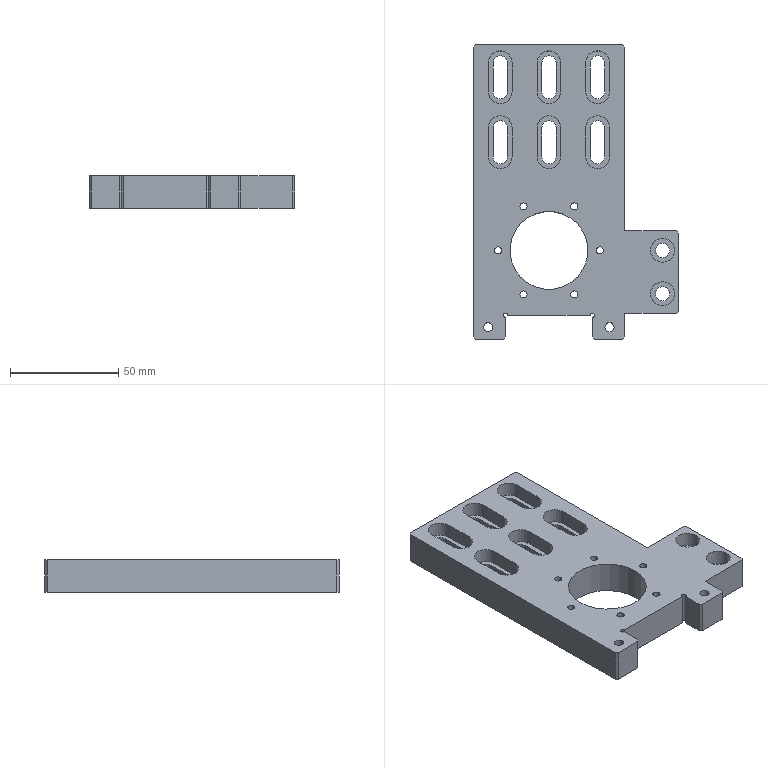Part | SolidWorks | features BaseBody 1 | 1 solid | 107 faces | box 95 x 136 x 15 mm | volume 116086 mm3 | plane 54 | cylinder 53 | commonest cylinder face diameters 6.6 x16 11 x16 3.3 x12 4.2 x4 2 x3 36 x2